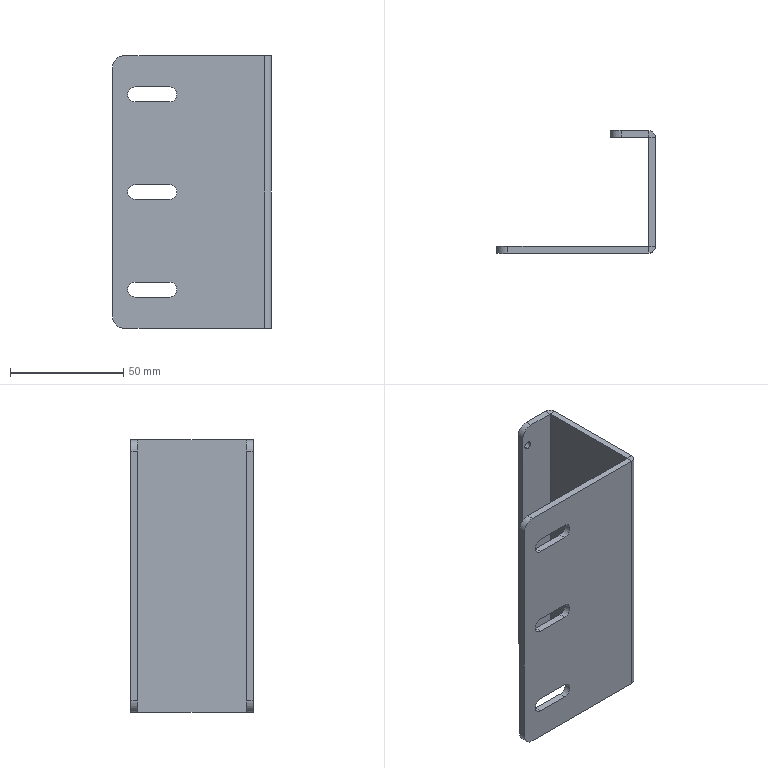Part | SolidWorks | features 3DProfileFeature 1, Fillet 1, FlatPattern 1, HoleWzd 1, ICE 1, SMBaseFlange 1, SheetMetal 1 | 1 solid | 45 faces | box 70 x 54 x 120 mm | volume 47871 mm3 | plane 24 | cylinder 21 | commonest cylinder face diameters 6.6 x9 3.4 x6 10 x4 6 x2
STEP:
#1=CARTESIAN_POINT('',(-17.,51.,8.3));
#2=VERTEX_POINT('',#1);
#3=CARTESIAN_POINT('',(-17.,51.,11.7));
#4=VERTEX_POINT('',#3);
#5=CARTESIAN_POINT('',(-17.,51.,10.));
#6=DIRECTION('',(0.,1.,0.));
#7=DIRECTION('',(0.,0.,1.));
#8=AXIS2_PLACEMENT_3D('',#5,#6,#7);
#9=CIRCLE('',#8,1.7);
#10=EDGE_CURVE('',#2,#4,#9,.T.);
#11=ORIENTED_EDGE('',*,*,#10,.F.);
#12=CARTESIAN_POINT('',(-17.,54.,8.3));
#13=VERTEX_POINT('',#12);
#14=CARTESIAN_POINT('',(-17.,54.,8.3));
#15=DIRECTION('',(0.,1.,0.));
#16=VECTOR('',#15,1000.);
#17=LINE('',#14,#16);
#18=EDGE_CURVE('',#2,#13,#17,.T.);
#19=ORIENTED_EDGE('',*,*,#18,.T.);
#20=CARTESIAN_POINT('',(-17.,54.,11.7));
#21=VERTEX_POINT('',#20);
#22=CARTESIAN_POINT('',(-17.,54.,10.));
#23=DIRECTION('',(0.,1.,0.));
#24=DIRECTION('',(0.,0.,1.));
#25=AXIS2_PLACEMENT_3D('',#22,#23,#24);
#26=CIRCLE('',#25,1.7);
#27=EDGE_CURVE('',#13,#21,#26,.T.);
#28=ORIENTED_EDGE('',*,*,#27,.T.);
#29=CARTESIAN_POINT('',(-17.,54.,11.7));
#30=DIRECTION('',(0.,1.,0.));
#31=VECTOR('',#30,1000.);
#32=LINE('',#29,#31);
#33=EDGE_CURVE('',#4,#21,#32,.T.);
#34=ORIENTED_EDGE('',*,*,#33,.F.);
#35=EDGE_LOOP('',(#11,#19,#28,#34));
#36=FACE_OUTER_BOUND('',#35,.T.);
#37=CARTESIAN_POINT('',(-17.,54.,10.));
#38=DIRECTION('',(0.,1.,0.));
#39=DIRECTION('',(0.,0.,1.));
#40=AXIS2_PLACEMENT_3D('',#37,#38,#39);
#41=CYLINDRICAL_SURFACE('',#40,1.7);
#42=ADVANCED_FACE('',(#36),#41,.F.);
#43=CARTESIAN_POINT('',(-17.,51.,58.3));
#44=VERTEX_POINT('',#43);
#45=CARTESIAN_POINT('',(-17.,51.,61.7));
#46=VERTEX_POINT('',#45);
#47=CARTESIAN_POINT('',(-17.,51.,60.));
#48=DIRECTION('',(0.,1.,0.));
#49=DIRECTION('',(0.,0.,1.));
#50=AXIS2_PLACEMENT_3D('',#47,#48,#49);
#51=CIRCLE('',#50,1.7);
#52=EDGE_CURVE('',#44,#46,#51,.T.);
#53=ORIENTED_EDGE('',*,*,#52,.F.);
#54=CARTESIAN_POINT('',(-17.,54.,58.3));
#55=VERTEX_POINT('',#54);
#56=CARTESIAN_POINT('',(-17.,54.,58.3));
#57=DIRECTION('',(0.,1.,0.));
#58=VECTOR('',#57,1000.);
#59=LINE('',#56,#58);
#60=EDGE_CURVE('',#44,#55,#59,.T.);
#61=ORIENTED_EDGE('',*,*,#60,.T.);
#62=CARTESIAN_POINT('',(-17.,54.,61.7));
#63=VERTEX_POINT('',#62);
#64=CARTESIAN_POINT('',(-17.,54.,60.));
#65=DIRECTION('',(0.,1.,0.));
#66=DIRECTION('',(0.,0.,1.));
#67=AXIS2_PLACEMENT_3D('',#64,#65,#66);
#68=CIRCLE('',#67,1.7);
#69=EDGE_CURVE('',#55,#63,#68,.T.);
#70=ORIENTED_EDGE('',*,*,#69,.T.);
#71=CARTESIAN_POINT('',(-17.,54.,61.7));
#72=DIRECTION('',(0.,1.,0.));
#73=VECTOR('',#72,1000.);
#74=LINE('',#71,#73);
#75=EDGE_CURVE('',#46,#63,#74,.T.);
#76=ORIENTED_EDGE('',*,*,#75,.F.);
#77=EDGE_LOOP('',(#53,#61,#70,#76));
#78=FACE_OUTER_BOUND('',#77,.T.);
#79=CARTESIAN_POINT('',(-17.,54.,60.));
#80=DIRECTION('',(0.,1.,0.));
#81=DIRECTION('',(0.,0.,1.));
#82=AXIS2_PLACEMENT_3D('',#79,#80,#81);
#83=CYLINDRICAL_SURFACE('',#82,1.7);
#84=ADVANCED_FACE('',(#78),#83,.F.);
#85=CARTESIAN_POINT('',(-17.,51.,108.3));
#86=VERTEX_POINT('',#85);
#87=CARTESIAN_POINT('',(-17.,51.,111.7));
#88=VERTEX_POINT('',#87);
#89=CARTESIAN_POINT('',(-17.,51.,110.));
#90=DIRECTION('',(0.,1.,0.));
#91=DIRECTION('',(0.,0.,1.));
#92=AXIS2_PLACEMENT_3D('',#89,#90,#91);
#93=CIRCLE('',#92,1.7);
#94=EDGE_CURVE('',#86,#88,#93,.T.);
#95=ORIENTED_EDGE('',*,*,#94,.F.);
#96=CARTESIAN_POINT('',(-17.,54.,108.3));
#97=VERTEX_POINT('',#96);
#98=CARTESIAN_POINT('',(-17.,54.,108.3));
#99=DIRECTION('',(0.,1.,0.));
#100=VECTOR('',#99,1000.);
#101=LINE('',#98,#100);
#102=EDGE_CURVE('',#86,#97,#101,.T.);
#103=ORIENTED_EDGE('',*,*,#102,.T.);
#104=CARTESIAN_POINT('',(-17.,54.,111.7));
#105=VERTEX_POINT('',#104);
#106=CARTESIAN_POINT('',(-17.,54.,110.));
#107=DIRECTION('',(0.,1.,0.));
#108=DIRECTION('',(0.,0.,1.));
#109=AXIS2_PLACEMENT_3D('',#106,#107,#108);
#110=CIRCLE('',#109,1.7);
#111=EDGE_CURVE('',#97,#105,#110,.T.);
#112=ORIENTED_EDGE('',*,*,#111,.T.);
#113=CARTESIAN_POINT('',(-17.,54.,111.7));
#114=DIRECTION('',(0.,1.,0.));
#115=VECTOR('',#114,1000.);
#116=LINE('',#113,#115);
#117=EDGE_CURVE('',#88,#105,#116,.T.);
#118=ORIENTED_EDGE('',*,*,#117,.F.);
#119=EDGE_LOOP('',(#95,#103,#112,#118));
#120=FACE_OUTER_BOUND('',#119,.T.);
#121=CARTESIAN_POINT('',(-17.,54.,110.));
#122=DIRECTION('',(0.,1.,0.));
#123=DIRECTION('',(0.,0.,1.));
#124=AXIS2_PLACEMENT_3D('',#121,#122,#123);
#125=CYLINDRICAL_SURFACE('',#124,1.7);
#126=ADVANCED_FACE('',(#120),#125,.F.);
#127=CARTESIAN_POINT('',(-63.3,0.,17.));
#128=VERTEX_POINT('',#127);
#129=CARTESIAN_POINT('',(-60.,0.,20.3));
#130=VERTEX_POINT('',#129);
#131=CARTESIAN_POINT('',(-60.,0.,17.));
#132=DIRECTION('',(0.,1.,0.));
#133=DIRECTION('',(-1.,0.,0.));
#134=AXIS2_PLACEMENT_3D('',#131,#132,#133);
#135=CIRCLE('',#134,3.3);
#136=EDGE_CURVE('',#128,#130,#135,.T.);
#137=ORIENTED_EDGE('',*,*,#136,.F.);
#138=CARTESIAN_POINT('',(-63.3,3.,17.));
#139=VERTEX_POINT('',#138);
#140=CARTESIAN_POINT('',(-63.3,0.,17.));
#141=DIRECTION('',(0.,1.,0.));
#142=VECTOR('',#141,1000.);
#143=LINE('',#140,#142);
#144=EDGE_CURVE('',#128,#139,#143,.T.);
#145=ORIENTED_EDGE('',*,*,#144,.T.);
#146=CARTESIAN_POINT('',(-60.,3.,20.3));
#147=VERTEX_POINT('',#146);
#148=CARTESIAN_POINT('',(-60.,3.,17.));
#149=DIRECTION('',(0.,1.,0.));
#150=DIRECTION('',(-1.,0.,0.));
#151=AXIS2_PLACEMENT_3D('',#148,#149,#150);
#152=CIRCLE('',#151,3.3);
#153=EDGE_CURVE('',#139,#147,#152,.T.);
#154=ORIENTED_EDGE('',*,*,#153,.T.);
#155=CARTESIAN_POINT('',(-60.,0.,20.3));
#156=DIRECTION('',(0.,1.,0.));
#157=VECTOR('',#156,1000.);
#158=LINE('',#155,#157);
#159=EDGE_CURVE('',#130,#147,#158,.T.);
#160=ORIENTED_EDGE('',*,*,#159,.F.);
#161=EDGE_LOOP('',(#137,#145,#154,#160));
#162=FACE_OUTER_BOUND('',#161,.T.);
#163=CARTESIAN_POINT('',(-60.,0.,17.));
#164=DIRECTION('',(0.,1.,0.));
#165=DIRECTION('',(-1.,0.,0.));
#166=AXIS2_PLACEMENT_3D('',#163,#164,#165);
#167=CYLINDRICAL_SURFACE('',#166,3.3);
#168=ADVANCED_FACE('',(#162),#167,.F.);
#169=CARTESIAN_POINT('',(-63.3,0.,60.));
#170=VERTEX_POINT('',#169);
#171=CARTESIAN_POINT('',(-60.,0.,63.3));
#172=VERTEX_POINT('',#171);
#173=CARTESIAN_POINT('',(-60.,0.,60.));
#174=DIRECTION('',(0.,1.,0.));
#175=DIRECTION('',(-1.,0.,0.));
#176=AXIS2_PLACEMENT_3D('',#173,#174,#175);
#177=CIRCLE('',#176,3.3);
#178=EDGE_CURVE('',#170,#172,#177,.T.);
#179=ORIENTED_EDGE('',*,*,#178,.F.);
#180=CARTESIAN_POINT('',(-63.3,3.,60.));
#181=VERTEX_POINT('',#180);
#182=CARTESIAN_POINT('',(-63.3,0.,60.));
#183=DIRECTION('',(0.,1.,0.));
#184=VECTOR('',#183,1000.);
#185=LINE('',#182,#184);
#186=EDGE_CURVE('',#170,#181,#185,.T.);
#187=ORIENTED_EDGE('',*,*,#186,.T.);
#188=CARTESIAN_POINT('',(-60.,3.,63.3));
#189=VERTEX_POINT('',#188);
#190=CARTESIAN_POINT('',(-60.,3.,60.));
#191=DIRECTION('',(0.,1.,0.));
#192=DIRECTION('',(-1.,0.,0.));
#193=AXIS2_PLACEMENT_3D('',#190,#191,#192);
#194=CIRCLE('',#193,3.3);
#195=EDGE_CURVE('',#181,#189,#194,.T.);
#196=ORIENTED_EDGE('',*,*,#195,.T.);
#197=CARTESIAN_POINT('',(-60.,0.,63.3));
#198=DIRECTION('',(0.,1.,0.));
#199=VECTOR('',#198,1000.);
#200=LINE('',#197,#199);
#201=EDGE_CURVE('',#172,#189,#200,.T.);
#202=ORIENTED_EDGE('',*,*,#201,.F.);
#203=EDGE_LOOP('',(#179,#187,#196,#202));
#204=FACE_OUTER_BOUND('',#203,.T.);
#205=CARTESIAN_POINT('',(-60.,0.,60.));
#206=DIRECTION('',(0.,1.,0.));
#207=DIRECTION('',(-1.,0.,0.));
#208=AXIS2_PLACEMENT_3D('',#205,#206,#207);
#209=CYLINDRICAL_SURFACE('',#208,3.3);
#210=ADVANCED_FACE('',(#204),#209,.F.);
#211=CARTESIAN_POINT('',(-63.3,0.,103.));
#212=VERTEX_POINT('',#211);
#213=CARTESIAN_POINT('',(-60.,0.,106.3));
#214=VERTEX_POINT('',#213);
#215=CARTESIAN_POINT('',(-60.,0.,103.));
#216=DIRECTION('',(0.,1.,0.));
#217=DIRECTION('',(-1.,0.,0.));
#218=AXIS2_PLACEMENT_3D('',#215,#216,#217);
#219=CIRCLE('',#218,3.3);
#220=EDGE_CURVE('',#212,#214,#219,.T.);
#221=ORIENTED_EDGE('',*,*,#220,.F.);
#222=CARTESIAN_POINT('',(-63.3,3.,103.));
#223=VERTEX_POINT('',#222);
#224=CARTESIAN_POINT('',(-63.3,0.,103.));
#225=DIRECTION('',(0.,1.,0.));
#226=VECTOR('',#225,1000.);
#227=LINE('',#224,#226);
#228=EDGE_CURVE('',#212,#223,#227,.T.);
#229=ORIENTED_EDGE('',*,*,#228,.T.);
#230=CARTESIAN_POINT('',(-60.,3.,106.3));
#231=VERTEX_POINT('',#230);
#232=CARTESIAN_POINT('',(-60.,3.,103.));
#233=DIRECTION('',(0.,1.,0.));
#234=DIRECTION('',(-1.,0.,0.));
#235=AXIS2_PLACEMENT_3D('',#232,#233,#234);
#236=CIRCLE('',#235,3.3);
#237=EDGE_CURVE('',#223,#231,#236,.T.);
#238=ORIENTED_EDGE('',*,*,#237,.T.);
#239=CARTESIAN_POINT('',(-60.,0.,106.3));
#240=DIRECTION('',(0.,1.,0.));
#241=VECTOR('',#240,1000.);
#242=LINE('',#239,#241);
#243=EDGE_CURVE('',#214,#231,#242,.T.);
#244=ORIENTED_EDGE('',*,*,#243,.F.);
#245=EDGE_LOOP('',(#221,#229,#238,#244));
#246=FACE_OUTER_BOUND('',#245,.T.);
#247=CARTESIAN_POINT('',(-60.,0.,103.));
#248=DIRECTION('',(0.,1.,0.));
#249=DIRECTION('',(-1.,0.,0.));
#250=AXIS2_PLACEMENT_3D('',#247,#248,#249);
#251=CYLINDRICAL_SURFACE('',#250,3.3);
#252=ADVANCED_FACE('',(#246),#251,.F.);
#253=CARTESIAN_POINT('',(-3.,51.,120.));
#254=VERTEX_POINT('',#253);
#255=CARTESIAN_POINT('',(0.,51.,120.));
#256=VERTEX_POINT('',#255);
#257=CARTESIAN_POINT('',(-3.,51.,120.));
#258=DIRECTION('',(1.,0.,0.));
#259=VECTOR('',#258,1000.);
#260=LINE('',#257,#259);
#261=EDGE_CURVE('',#254,#256,#260,.T.);
#262=ORIENTED_EDGE('',*,*,#261,.F.);
#263=CARTESIAN_POINT('',(-3.,3.,120.));
#264=VERTEX_POINT('',#263);
#265=CARTESIAN_POINT('',(-3.,0.,120.));
#266=DIRECTION('',(0.,-1.,0.));
#267=VECTOR('',#266,1000.);
#268=LINE('',#265,#267);
#269=EDGE_CURVE('',#254,#264,#268,.T.);
#270=ORIENTED_EDGE('',*,*,#269,.T.);
#271=CARTESIAN_POINT('',(0.,3.,120.));
#272=VERTEX_POINT('',#271);
#273=CARTESIAN_POINT('',(-3.,3.,120.));
#274=DIRECTION('',(1.,0.,0.));
#275=VECTOR('',#274,1000.);
#276=LINE('',#273,#275);
#277=EDGE_CURVE('',#264,#272,#276,.T.);
#278=ORIENTED_EDGE('',*,*,#277,.T.);
#279=CARTESIAN_POINT('',(0.,0.,120.));
#280=DIRECTION('',(0.,-1.,0.));
#281=VECTOR('',#280,1000.);
#282=LINE('',#279,#281);
#283=EDGE_CURVE('',#256,#272,#282,.T.);
#284=ORIENTED_EDGE('',*,*,#283,.F.);
#285=EDGE_LOOP('',(#262,#270,#278,#284));
#286=FACE_OUTER_BOUND('',#285,.T.);
#287=CARTESIAN_POINT('',(-3.,51.,120.));
#288=DIRECTION('',(0.,0.,1.));
#289=DIRECTION('',(1.,0.,0.));
#290=AXIS2_PLACEMENT_3D('',#287,#288,#289);
#291=PLANE('',#290);
#292=ADVANCED_FACE('',(#286),#291,.T.);
#293=CARTESIAN_POINT('',(-3.,54.,120.));
#294=VERTEX_POINT('',#293);
#295=CARTESIAN_POINT('',(-3.,51.,120.));
#296=DIRECTION('',(0.,1.,0.));
#297=VECTOR('',#296,1000.);
#298=LINE('',#295,#297);
#299=EDGE_CURVE('',#254,#294,#298,.T.);
#300=ORIENTED_EDGE('',*,*,#299,.F.);
#301=ORIENTED_EDGE('',*,*,#261,.T.);
#302=CARTESIAN_POINT('',(-3.,51.,120.));
#303=DIRECTION('',(0.,0.,-1.));
#304=DIRECTION('',(1.,0.,0.));
#305=AXIS2_PLACEMENT_3D('',#302,#303,#304);
#306=CIRCLE('',#305,3.);
#307=EDGE_CURVE('',#294,#256,#306,.T.);
#308=ORIENTED_EDGE('',*,*,#307,.F.);
#309=EDGE_LOOP('',(#300,#301,#308));
#310=FACE_OUTER_BOUND('',#309,.T.);
#311=CARTESIAN_POINT('',(-3.,51.,120.));
#312=DIRECTION('',(0.,0.,1.));
#313=DIRECTION('',(1.,0.,0.));
#314=AXIS2_PLACEMENT_3D('',#311,#312,#313);
#315=PLANE('',#314);
#316=ADVANCED_FACE('',(#310),#315,.T.);
#317=CARTESIAN_POINT('',(-15.,51.,0.));
#318=VERTEX_POINT('',#317);
#319=CARTESIAN_POINT('',(-3.,51.,0.));
#320=VERTEX_POINT('',#319);
#321=CARTESIAN_POINT('',(0.,51.,0.));
#322=DIRECTION('',(1.,0.,0.));
#323=VECTOR('',#322,1000.);
#324=LINE('',#321,#323);
#325=EDGE_CURVE('',#318,#320,#324,.T.);
#326=ORIENTED_EDGE('',*,*,#325,.F.);
#327=CARTESIAN_POINT('',(-15.,54.,0.));
#328=VERTEX_POINT('',#327);
#329=CARTESIAN_POINT('',(-15.,51.,0.));
#330=DIRECTION('',(0.,1.,0.));
#331=VECTOR('',#330,1000.);
#332=LINE('',#329,#331);
#333=EDGE_CURVE('',#318,#328,#332,.T.);
#334=ORIENTED_EDGE('',*,*,#333,.T.);
#335=CARTESIAN_POINT('',(-3.,54.,0.));
#336=VERTEX_POINT('',#335);
#337=CARTESIAN_POINT('',(0.,54.,0.));
#338=DIRECTION('',(1.,0.,0.));
#339=VECTOR('',#338,1000.);
#340=LINE('',#337,#339);
#341=EDGE_CURVE('',#328,#336,#340,.T.);
#342=ORIENTED_EDGE('',*,*,#341,.T.);
#343=CARTESIAN_POINT('',(-3.,51.,0.));
#344=DIRECTION('',(0.,1.,0.));
#345=VECTOR('',#344,1000.);
#346=LINE('',#343,#345);
#347=EDGE_CURVE('',#320,#336,#346,.T.);
#348=ORIENTED_EDGE('',*,*,#347,.F.);
#349=EDGE_LOOP('',(#326,#334,#342,#348));
#350=FACE_OUTER_BOUND('',#349,.T.);
#351=CARTESIAN_POINT('',(-3.,51.,0.));
#352=DIRECTION('',(0.,0.,-1.));
#353=DIRECTION('',(-1.,0.,0.));
#354=AXIS2_PLACEMENT_3D('',#351,#352,#353);
#355=PLANE('',#354);
#356=ADVANCED_FACE('',(#350),#355,.T.);
#357=CARTESIAN_POINT('',(0.,51.,0.));
#358=VERTEX_POINT('',#357);
#359=CARTESIAN_POINT('',(-3.,51.,0.));
#360=DIRECTION('',(1.,0.,0.));
#361=VECTOR('',#360,1000.);
#362=LINE('',#359,#361);
#363=EDGE_CURVE('',#320,#358,#362,.T.);
#364=ORIENTED_EDGE('',*,*,#363,.F.);
#365=ORIENTED_EDGE('',*,*,#347,.T.);
#366=CARTESIAN_POINT('',(-3.,51.,0.));
#367=DIRECTION('',(0.,0.,-1.));
#368=DIRECTION('',(1.,0.,0.));
#369=AXIS2_PLACEMENT_3D('',#366,#367,#368);
#370=CIRCLE('',#369,3.);
#371=EDGE_CURVE('',#336,#358,#370,.T.);
#372=ORIENTED_EDGE('',*,*,#371,.T.);
#373=EDGE_LOOP('',(#364,#365,#372));
#374=FACE_OUTER_BOUND('',#373,.T.);
#375=CARTESIAN_POINT('',(-3.,51.,0.));
#376=DIRECTION('',(0.,0.,-1.));
#377=DIRECTION('',(-1.,0.,0.));
#378=AXIS2_PLACEMENT_3D('',#375,#376,#377);
#379=PLANE('',#378);
#380=ADVANCED_FACE('',(#374),#379,.T.);
#381=CARTESIAN_POINT('',(-65.,3.,120.));
#382=VERTEX_POINT('',#381);
#383=CARTESIAN_POINT('',(0.,3.,120.));
#384=DIRECTION('',(-1.,0.,0.));
#385=VECTOR('',#384,1000.);
#386=LINE('',#383,#385);
#387=EDGE_CURVE('',#264,#382,#386,.T.);
#388=ORIENTED_EDGE('',*,*,#387,.T.);
#389=CARTESIAN_POINT('',(-65.,0.,120.));
#390=VERTEX_POINT('',#389);
#391=CARTESIAN_POINT('',(-65.,3.,120.));
#392=DIRECTION('',(0.,-1.,0.));
#393=VECTOR('',#392,1000.);
#394=LINE('',#391,#393);
#395=EDGE_CURVE('',#382,#390,#394,.T.);
#396=ORIENTED_EDGE('',*,*,#395,.T.);
#397=CARTESIAN_POINT('',(-3.,0.,120.));
#398=VERTEX_POINT('',#397);
#399=CARTESIAN_POINT('',(0.,0.,120.));
#400=DIRECTION('',(-1.,0.,0.));
#401=VECTOR('',#400,1000.);
#402=LINE('',#399,#401);
#403=EDGE_CURVE('',#398,#390,#402,.T.);
#404=ORIENTED_EDGE('',*,*,#403,.F.);
#405=CARTESIAN_POINT('',(-3.,3.,120.));
#406=DIRECTION('',(0.,-1.,0.));
#407=VECTOR('',#406,1000.);
#408=LINE('',#405,#407);
#409=EDGE_CURVE('',#264,#398,#408,.T.);
#410=ORIENTED_EDGE('',*,*,#409,.F.);
#411=EDGE_LOOP('',(#388,#396,#404,#410));
#412=FACE_OUTER_BOUND('',#411,.T.);
#413=CARTESIAN_POINT('',(-3.,3.,120.));
#414=DIRECTION('',(0.,0.,1.));
#415=DIRECTION('',(1.,0.,0.));
#416=AXIS2_PLACEMENT_3D('',#413,#414,#415);
#417=PLANE('',#416);
#418=ADVANCED_FACE('',(#412),#417,.T.);
#419=ORIENTED_EDGE('',*,*,#277,.F.);
#420=ORIENTED_EDGE('',*,*,#409,.T.);
#421=CARTESIAN_POINT('',(-3.,3.,120.));
#422=DIRECTION('',(0.,0.,-1.));
#423=DIRECTION('',(1.,0.,0.));
#424=AXIS2_PLACEMENT_3D('',#421,#422,#423);
#425=CIRCLE('',#424,3.);
#426=EDGE_CURVE('',#272,#398,#425,.T.);
#427=ORIENTED_EDGE('',*,*,#426,.F.);
#428=EDGE_LOOP('',(#419,#420,#427));
#429=FACE_OUTER_BOUND('',#428,.T.);
#430=CARTESIAN_POINT('',(-3.,3.,120.));
#431=DIRECTION('',(0.,0.,1.));
#432=DIRECTION('',(1.,0.,0.));
#433=AXIS2_PLACEMENT_3D('',#430,#431,#432);
#434=PLANE('',#433);
#435=ADVANCED_FACE('',(#429),#434,.T.);
#436=CARTESIAN_POINT('',(-3.,3.,0.));
#437=VERTEX_POINT('',#436);
#438=CARTESIAN_POINT('',(0.,3.,0.));
#439=VERTEX_POINT('',#438);
#440=CARTESIAN_POINT('',(-3.,3.,0.));
#441=DIRECTION('',(1.,0.,0.));
#442=VECTOR('',#441,1000.);
#443=LINE('',#440,#442);
#444=EDGE_CURVE('',#437,#439,#443,.T.);
#445=ORIENTED_EDGE('',*,*,#444,.F.);
#446=CARTESIAN_POINT('',(-3.,0.,0.));
#447=DIRECTION('',(0.,-1.,0.));
#448=VECTOR('',#447,1000.);
#449=LINE('',#446,#448);
#450=EDGE_CURVE('',#320,#437,#449,.T.);
#451=ORIENTED_EDGE('',*,*,#450,.F.);
#452=ORIENTED_EDGE('',*,*,#363,.T.);
#453=CARTESIAN_POINT('',(0.,0.,0.));
#454=DIRECTION('',(0.,-1.,0.));
#455=VECTOR('',#454,1000.);
#456=LINE('',#453,#455);
#457=EDGE_CURVE('',#358,#439,#456,.T.);
#458=ORIENTED_EDGE('',*,*,#457,.T.);
#459=EDGE_LOOP('',(#445,#451,#452,#458));
#460=FACE_OUTER_BOUND('',#459,.T.);
#461=CARTESIAN_POINT('',(-3.,3.,0.));
#462=DIRECTION('',(0.,0.,-1.));
#463=DIRECTION('',(-1.,0.,0.));
#464=AXIS2_PLACEMENT_3D('',#461,#462,#463);
#465=PLANE('',#464);
#466=ADVANCED_FACE('',(#460),#465,.T.);
#467=CARTESIAN_POINT('',(-3.,0.,0.));
#468=VERTEX_POINT('',#467);
#469=CARTESIAN_POINT('',(-3.,3.,0.));
#470=DIRECTION('',(0.,-1.,0.));
#471=VECTOR('',#470,1000.);
#472=LINE('',#469,#471);
#473=EDGE_CURVE('',#437,#468,#472,.T.);
#474=ORIENTED_EDGE('',*,*,#473,.F.);
#475=ORIENTED_EDGE('',*,*,#444,.T.);
#476=CARTESIAN_POINT('',(-3.,3.,0.));
#477=DIRECTION('',(0.,0.,-1.));
#478=DIRECTION('',(1.,0.,0.));
#479=AXIS2_PLACEMENT_3D('',#476,#477,#478);
#480=CIRCLE('',#479,3.);
#481=EDGE_CURVE('',#439,#468,#480,.T.);
#482=ORIENTED_EDGE('',*,*,#481,.T.);
#483=EDGE_LOOP('',(#474,#475,#482));
#484=FACE_OUTER_BOUND('',#483,.T.);
#485=CARTESIAN_POINT('',(-3.,3.,0.));
#486=DIRECTION('',(0.,0.,-1.));
#487=DIRECTION('',(-1.,0.,0.));
#488=AXIS2_PLACEMENT_3D('',#485,#486,#487);
#489=PLANE('',#488);
#490=ADVANCED_FACE('',(#484),#489,.T.);
#491=CARTESIAN_POINT('',(-45.,3.,20.3));
#492=VERTEX_POINT('',#491);
#493=CARTESIAN_POINT('',(-60.,3.,20.3));
#494=DIRECTION('',(1.,0.,0.));
#495=VECTOR('',#494,1000.);
#496=LINE('',#493,#495);
#497=EDGE_CURVE('',#147,#492,#496,.T.);
#498=ORIENTED_EDGE('',*,*,#497,.F.);
#499=ORIENTED_EDGE('',*,*,#153,.F.);
#500=CARTESIAN_POINT('',(-60.,3.,13.7));
#501=VERTEX_POINT('',#500);
#502=CARTESIAN_POINT('',(-60.,3.,17.));
#503=DIRECTION('',(0.,1.,0.));
#504=DIRECTION('',(-1.,0.,0.));
#505=AXIS2_PLACEMENT_3D('',#502,#503,#504);
#506=CIRCLE('',#505,3.3);
#507=EDGE_CURVE('',#501,#139,#506,.T.);
#508=ORIENTED_EDGE('',*,*,#507,.F.);
#509=CARTESIAN_POINT('',(-45.,3.,13.7));
#510=VERTEX_POINT('',#509);
#511=CARTESIAN_POINT('',(-60.,3.,13.7));
#512=DIRECTION('',(-1.,0.,0.));
#513=VECTOR('',#512,1000.);
#514=LINE('',#511,#513);
#515=EDGE_CURVE('',#510,#501,#514,.T.);
#516=ORIENTED_EDGE('',*,*,#515,.F.);
#517=CARTESIAN_POINT('',(-45.,3.,17.));
#518=DIRECTION('',(0.,1.,0.));
#519=DIRECTION('',(-1.,0.,0.));
#520=AXIS2_PLACEMENT_3D('',#517,#518,#519);
#521=CIRCLE('',#520,3.3);
#522=EDGE_CURVE('',#492,#510,#521,.T.);
#523=ORIENTED_EDGE('',*,*,#522,.F.);
#524=EDGE_LOOP('',(#498,#499,#508,#516,#523));
#525=FACE_BOUND('',#524,.T.);
#526=CARTESIAN_POINT('',(-45.,3.,63.3));
#527=VERTEX_POINT('',#526);
#528=CARTESIAN_POINT('',(-60.,3.,63.3));
#529=DIRECTION('',(1.,0.,0.));
#530=VECTOR('',#529,1000.);
#531=LINE('',#528,#530);
#532=EDGE_CURVE('',#189,#527,#531,.T.);
#533=ORIENTED_EDGE('',*,*,#532,.F.);
#534=ORIENTED_EDGE('',*,*,#195,.F.);
#535=CARTESIAN_POINT('',(-60.,3.,56.7));
#536=VERTEX_POINT('',#535);
#537=CARTESIAN_POINT('',(-60.,3.,60.));
#538=DIRECTION('',(0.,1.,0.));
#539=DIRECTION('',(-1.,0.,0.));
#540=AXIS2_PLACEMENT_3D('',#537,#538,#539);
#541=CIRCLE('',#540,3.3);
#542=EDGE_CURVE('',#536,#181,#541,.T.);
#543=ORIENTED_EDGE('',*,*,#542,.F.);
#544=CARTESIAN_POINT('',(-45.,3.,56.7));
#545=VERTEX_POINT('',#544);
#546=CARTESIAN_POINT('',(-60.,3.,56.7));
#547=DIRECTION('',(-1.,0.,0.));
#548=VECTOR('',#547,1000.);
#549=LINE('',#546,#548);
#550=EDGE_CURVE('',#545,#536,#549,.T.);
#551=ORIENTED_EDGE('',*,*,#550,.F.);
#552=CARTESIAN_POINT('',(-45.,3.,60.));
#553=DIRECTION('',(0.,1.,0.));
#554=DIRECTION('',(-1.,0.,0.));
#555=AXIS2_PLACEMENT_3D('',#552,#553,#554);
#556=CIRCLE('',#555,3.3);
#557=EDGE_CURVE('',#527,#545,#556,.T.);
#558=ORIENTED_EDGE('',*,*,#557,.F.);
#559=EDGE_LOOP('',(#533,#534,#543,#551,#558));
#560=FACE_BOUND('',#559,.T.);
#561=CARTESIAN_POINT('',(-45.,3.,106.3));
#562=VERTEX_POINT('',#561);
#563=CARTESIAN_POINT('',(-60.,3.,106.3));
#564=DIRECTION('',(1.,0.,0.));
#565=VECTOR('',#564,1000.);
#566=LINE('',#563,#565);
#567=EDGE_CURVE('',#231,#562,#566,.T.);
#568=ORIENTED_EDGE('',*,*,#567,.F.);
#569=ORIENTED_EDGE('',*,*,#237,.F.);
#570=CARTESIAN_POINT('',(-60.,3.,99.7));
#571=VERTEX_POINT('',#570);
#572=CARTESIAN_POINT('',(-60.,3.,103.));
#573=DIRECTION('',(0.,1.,0.));
#574=DIRECTION('',(-1.,0.,0.));
#575=AXIS2_PLACEMENT_3D('',#572,#573,#574);
#576=CIRCLE('',#575,3.3);
#577=EDGE_CURVE('',#571,#223,#576,.T.);
#578=ORIENTED_EDGE('',*,*,#577,.F.);
#579=CARTESIAN_POINT('',(-45.,3.,99.7));
#580=VERTEX_POINT('',#579);
#581=CARTESIAN_POINT('',(-60.,3.,99.7));
#582=DIRECTION('',(-1.,0.,0.));
#583=VECTOR('',#582,1000.);
#584=LINE('',#581,#583);
#585=EDGE_CURVE('',#580,#571,#584,.T.);
#586=ORIENTED_EDGE('',*,*,#585,.F.);
#587=CARTESIAN_POINT('',(-45.,3.,103.));
#588=DIRECTION('',(0.,1.,0.));
#589=DIRECTION('',(-1.,0.,0.));
#590=AXIS2_PLACEMENT_3D('',#587,#588,#589);
#591=CIRCLE('',#590,3.3);
#592=EDGE_CURVE('',#562,#580,#591,.T.);
#593=ORIENTED_EDGE('',*,*,#592,.F.);
#594=EDGE_LOOP('',(#568,#569,#578,#586,#593));
#595=FACE_BOUND('',#594,.T.);
#596=CARTESIAN_POINT('',(-65.,3.,0.));
#597=VERTEX_POINT('',#596);
#598=CARTESIAN_POINT('',(0.,3.,0.));
#599=DIRECTION('',(-1.,0.,0.));
#600=VECTOR('',#599,1000.);
#601=LINE('',#598,#600);
#602=EDGE_CURVE('',#437,#597,#601,.T.);
#603=ORIENTED_EDGE('',*,*,#602,.T.);
#604=CARTESIAN_POINT('',(-70.,3.,5.));
#605=VERTEX_POINT('',#604);
#606=CARTESIAN_POINT('',(-65.,3.,5.));
#607=DIRECTION('',(0.,1.,0.));
#608=DIRECTION('',(1.,0.,0.));
#609=AXIS2_PLACEMENT_3D('',#606,#607,#608);
#610=CIRCLE('',#609,5.);
#611=EDGE_CURVE('',#597,#605,#610,.T.);
#612=ORIENTED_EDGE('',*,*,#611,.T.);
#613=CARTESIAN_POINT('',(-70.,3.,115.));
#614=VERTEX_POINT('',#613);
#615=CARTESIAN_POINT('',(-70.,3.,120.));
#616=DIRECTION('',(0.,0.,-1.));
#617=VECTOR('',#616,1000.);
#618=LINE('',#615,#617);
#619=EDGE_CURVE('',#614,#605,#618,.T.);
#620=ORIENTED_EDGE('',*,*,#619,.F.);
#621=CARTESIAN_POINT('',(-65.,3.,115.));
#622=DIRECTION('',(0.,1.,0.));
#623=DIRECTION('',(1.,0.,0.));
#624=AXIS2_PLACEMENT_3D('',#621,#622,#623);
#625=CIRCLE('',#624,5.);
#626=EDGE_CURVE('',#614,#382,#625,.T.);
#627=ORIENTED_EDGE('',*,*,#626,.T.);
#628=ORIENTED_EDGE('',*,*,#387,.F.);
#629=CARTESIAN_POINT('',(-3.,3.,120.));
#630=DIRECTION('',(0.,0.,-1.));
#631=VECTOR('',#630,1000.);
#632=LINE('',#629,#631);
#633=EDGE_CURVE('',#264,#437,#632,.T.);
#634=ORIENTED_EDGE('',*,*,#633,.T.);
#635=EDGE_LOOP('',(#603,#612,#620,#627,#628,#634));
#636=FACE_OUTER_BOUND('',#635,.T.);
#637=CARTESIAN_POINT('',(0.,3.,120.));
#638=DIRECTION('',(0.,-1.,0.));
#639=DIRECTION('',(1.,0.,0.));
#640=AXIS2_PLACEMENT_3D('',#637,#638,#639);
#641=PLANE('',#640);
#642=ADVANCED_FACE('',(#525,#560,#595,#636),#641,.F.);
#643=ORIENTED_EDGE('',*,*,#619,.T.);
#644=CARTESIAN_POINT('',(-70.,0.,5.));
#645=VERTEX_POINT('',#644);
#646=CARTESIAN_POINT('',(-70.,0.,5.));
#647=DIRECTION('',(0.,-1.,0.));
#648=VECTOR('',#647,1000.);
#649=LINE('',#646,#648);
#650=EDGE_CURVE('',#605,#645,#649,.T.);
#651=ORIENTED_EDGE('',*,*,#650,.T.);
#652=CARTESIAN_POINT('',(-70.,0.,115.));
#653=VERTEX_POINT('',#652);
#654=CARTESIAN_POINT('',(-70.,0.,120.));
#655=DIRECTION('',(0.,0.,-1.));
#656=VECTOR('',#655,1000.);
#657=LINE('',#654,#656);
#658=EDGE_CURVE('',#653,#645,#657,.T.);
#659=ORIENTED_EDGE('',*,*,#658,.F.);
#660=CARTESIAN_POINT('',(-70.,0.,115.));
#661=DIRECTION('',(0.,1.,0.));
#662=VECTOR('',#661,1000.);
#663=LINE('',#660,#662);
#664=EDGE_CURVE('',#653,#614,#663,.T.);
#665=ORIENTED_EDGE('',*,*,#664,.T.);
#666=EDGE_LOOP('',(#643,#651,#659,#665));
#667=FACE_OUTER_BOUND('',#666,.T.);
#668=CARTESIAN_POINT('',(-70.,0.,120.));
#669=DIRECTION('',(-1.,0.,0.));
#670=DIRECTION('',(0.,0.,1.));
#671=AXIS2_PLACEMENT_3D('',#668,#669,#670);
#672=PLANE('',#671);
#673=ADVANCED_FACE('',(#667),#672,.T.);
#674=CARTESIAN_POINT('',(-60.,0.,13.7));
#675=VERTEX_POINT('',#674);
#676=CARTESIAN_POINT('',(-60.,0.,17.));
#677=DIRECTION('',(0.,1.,0.));
#678=DIRECTION('',(-1.,0.,0.));
#679=AXIS2_PLACEMENT_3D('',#676,#677,#678);
#680=CIRCLE('',#679,3.3);
#681=EDGE_CURVE('',#675,#128,#680,.T.);
#682=ORIENTED_EDGE('',*,*,#681,.T.);
#683=ORIENTED_EDGE('',*,*,#136,.T.);
#684=CARTESIAN_POINT('',(-45.,0.,20.3));
#685=VERTEX_POINT('',#684);
#686=CARTESIAN_POINT('',(-60.,0.,20.3));
#687=DIRECTION('',(1.,0.,0.));
#688=VECTOR('',#687,1000.);
#689=LINE('',#686,#688);
#690=EDGE_CURVE('',#130,#685,#689,.T.);
#691=ORIENTED_EDGE('',*,*,#690,.T.);
#692=CARTESIAN_POINT('',(-45.,0.,13.7));
#693=VERTEX_POINT('',#692);
#694=CARTESIAN_POINT('',(-45.,0.,17.));
#695=DIRECTION('',(0.,1.,0.));
#696=DIRECTION('',(-1.,0.,0.));
#697=AXIS2_PLACEMENT_3D('',#694,#695,#696);
#698=CIRCLE('',#697,3.3);
#699=EDGE_CURVE('',#685,#693,#698,.T.);
#700=ORIENTED_EDGE('',*,*,#699,.T.);
#701=CARTESIAN_POINT('',(-60.,0.,13.7));
#702=DIRECTION('',(-1.,0.,0.));
#703=VECTOR('',#702,1000.);
#704=LINE('',#701,#703);
#705=EDGE_CURVE('',#693,#675,#704,.T.);
#706=ORIENTED_EDGE('',*,*,#705,.T.);
#707=EDGE_LOOP('',(#682,#683,#691,#700,#706));
#708=FACE_BOUND('',#707,.T.);
#709=CARTESIAN_POINT('',(-60.,0.,56.7));
#710=VERTEX_POINT('',#709);
#711=CARTESIAN_POINT('',(-60.,0.,60.));
#712=DIRECTION('',(0.,1.,0.));
#713=DIRECTION('',(-1.,0.,0.));
#714=AXIS2_PLACEMENT_3D('',#711,#712,#713);
#715=CIRCLE('',#714,3.3);
#716=EDGE_CURVE('',#710,#170,#715,.T.);
#717=ORIENTED_EDGE('',*,*,#716,.T.);
#718=ORIENTED_EDGE('',*,*,#178,.T.);
#719=CARTESIAN_POINT('',(-45.,0.,63.3));
#720=VERTEX_POINT('',#719);
#721=CARTESIAN_POINT('',(-60.,0.,63.3));
#722=DIRECTION('',(1.,0.,0.));
#723=VECTOR('',#722,1000.);
#724=LINE('',#721,#723);
#725=EDGE_CURVE('',#172,#720,#724,.T.);
#726=ORIENTED_EDGE('',*,*,#725,.T.);
#727=CARTESIAN_POINT('',(-45.,0.,56.7));
#728=VERTEX_POINT('',#727);
#729=CARTESIAN_POINT('',(-45.,0.,60.));
#730=DIRECTION('',(0.,1.,0.));
#731=DIRECTION('',(-1.,0.,0.));
#732=AXIS2_PLACEMENT_3D('',#729,#730,#731);
#733=CIRCLE('',#732,3.3);
#734=EDGE_CURVE('',#720,#728,#733,.T.);
#735=ORIENTED_EDGE('',*,*,#734,.T.);
#736=CARTESIAN_POINT('',(-60.,0.,56.7));
#737=DIRECTION('',(-1.,0.,0.));
#738=VECTOR('',#737,1000.);
#739=LINE('',#736,#738);
#740=EDGE_CURVE('',#728,#710,#739,.T.);
#741=ORIENTED_EDGE('',*,*,#740,.T.);
#742=EDGE_LOOP('',(#717,#718,#726,#735,#741));
#743=FACE_BOUND('',#742,.T.);
#744=CARTESIAN_POINT('',(-60.,0.,99.7));
#745=VERTEX_POINT('',#744);
#746=CARTESIAN_POINT('',(-60.,0.,103.));
#747=DIRECTION('',(0.,1.,0.));
#748=DIRECTION('',(-1.,0.,0.));
#749=AXIS2_PLACEMENT_3D('',#746,#747,#748);
#750=CIRCLE('',#749,3.3);
#751=EDGE_CURVE('',#745,#212,#750,.T.);
#752=ORIENTED_EDGE('',*,*,#751,.T.);
#753=ORIENTED_EDGE('',*,*,#220,.T.);
#754=CARTESIAN_POINT('',(-45.,0.,106.3));
#755=VERTEX_POINT('',#754);
#756=CARTESIAN_POINT('',(-60.,0.,106.3));
#757=DIRECTION('',(1.,0.,0.));
#758=VECTOR('',#757,1000.);
#759=LINE('',#756,#758);
#760=EDGE_CURVE('',#214,#755,#759,.T.);
#761=ORIENTED_EDGE('',*,*,#760,.T.);
#762=CARTESIAN_POINT('',(-45.,0.,99.7));
#763=VERTEX_POINT('',#762);
#764=CARTESIAN_POINT('',(-45.,0.,103.));
#765=DIRECTION('',(0.,1.,0.));
#766=DIRECTION('',(-1.,0.,0.));
#767=AXIS2_PLACEMENT_3D('',#764,#765,#766);
#768=CIRCLE('',#767,3.3);
#769=EDGE_CURVE('',#755,#763,#768,.T.);
#770=ORIENTED_EDGE('',*,*,#769,.T.);
#771=CARTESIAN_POINT('',(-60.,0.,99.7));
#772=DIRECTION('',(-1.,0.,0.));
#773=VECTOR('',#772,1000.);
#774=LINE('',#771,#773);
#775=EDGE_CURVE('',#763,#745,#774,.T.);
#776=ORIENTED_EDGE('',*,*,#775,.T.);
#777=EDGE_LOOP('',(#752,#753,#761,#770,#776));
#778=FACE_BOUND('',#777,.T.);
#779=ORIENTED_EDGE('',*,*,#658,.T.);
#780=CARTESIAN_POINT('',(-65.,0.,0.));
#781=VERTEX_POINT('',#780);
#782=CARTESIAN_POINT('',(-65.,0.,5.));
#783=DIRECTION('',(0.,-1.,0.));
#784=DIRECTION('',(1.,0.,0.));
#785=AXIS2_PLACEMENT_3D('',#782,#783,#784);
#786=CIRCLE('',#785,5.);
#787=EDGE_CURVE('',#645,#781,#786,.T.);
#788=ORIENTED_EDGE('',*,*,#787,.T.);
#789=CARTESIAN_POINT('',(0.,0.,0.));
#790=DIRECTION('',(-1.,0.,0.));
#791=VECTOR('',#790,1000.);
#792=LINE('',#789,#791);
#793=EDGE_CURVE('',#468,#781,#792,.T.);
#794=ORIENTED_EDGE('',*,*,#793,.F.);
#795=CARTESIAN_POINT('',(-3.,0.,120.));
#796=DIRECTION('',(0.,0.,-1.));
#797=VECTOR('',#796,1000.);
#798=LINE('',#795,#797);
#799=EDGE_CURVE('',#398,#468,#798,.T.);
#800=ORIENTED_EDGE('',*,*,#799,.F.);
#801=ORIENTED_EDGE('',*,*,#403,.T.);
#802=CARTESIAN_POINT('',(-65.,0.,115.));
#803=DIRECTION('',(0.,-1.,0.));
#804=DIRECTION('',(1.,0.,0.));
#805=AXIS2_PLACEMENT_3D('',#802,#803,#804);
#806=CIRCLE('',#805,5.);
#807=EDGE_CURVE('',#390,#653,#806,.T.);
#808=ORIENTED_EDGE('',*,*,#807,.T.);
#809=EDGE_LOOP('',(#779,#788,#794,#800,#801,#808));
#810=FACE_OUTER_BOUND('',#809,.T.);
#811=CARTESIAN_POINT('',(0.,0.,120.));
#812=DIRECTION('',(0.,-1.,0.));
#813=DIRECTION('',(1.,0.,0.));
#814=AXIS2_PLACEMENT_3D('',#811,#812,#813);
#815=PLANE('',#814);
#816=ADVANCED_FACE('',(#708,#743,#778,#810),#815,.T.);
#817=ORIENTED_EDGE('',*,*,#481,.F.);
#818=CARTESIAN_POINT('',(0.,3.,120.));
#819=DIRECTION('',(0.,0.,-1.));
#820=VECTOR('',#819,1000.);
#821=LINE('',#818,#820);
#822=EDGE_CURVE('',#272,#439,#821,.T.);
#823=ORIENTED_EDGE('',*,*,#822,.F.);
#824=ORIENTED_EDGE('',*,*,#426,.T.);
#825=ORIENTED_EDGE('',*,*,#799,.T.);
#826=EDGE_LOOP('',(#817,#823,#824,#825));
#827=FACE_OUTER_BOUND('',#826,.T.);
#828=CARTESIAN_POINT('',(-3.,3.,120.));
#829=DIRECTION('',(0.,0.,-1.));
#830=DIRECTION('',(-1.,0.,0.));
#831=AXIS2_PLACEMENT_3D('',#828,#829,#830);
#832=CYLINDRICAL_SURFACE('',#831,3.);
#833=ADVANCED_FACE('',(#827),#832,.T.);
#834=ORIENTED_EDGE('',*,*,#457,.F.);
#835=CARTESIAN_POINT('',(0.,51.,120.));
#836=DIRECTION('',(0.,0.,-1.));
#837=VECTOR('',#836,1000.);
#838=LINE('',#835,#837);
#839=EDGE_CURVE('',#256,#358,#838,.T.);
#840=ORIENTED_EDGE('',*,*,#839,.F.);
#841=ORIENTED_EDGE('',*,*,#283,.T.);
#842=ORIENTED_EDGE('',*,*,#822,.T.);
#843=EDGE_LOOP('',(#834,#840,#841,#842));
#844=FACE_OUTER_BOUND('',#843,.T.);
#845=CARTESIAN_POINT('',(0.,0.,120.));
#846=DIRECTION('',(1.,0.,0.));
#847=DIRECTION('',(0.,0.,-1.));
#848=AXIS2_PLACEMENT_3D('',#845,#846,#847);
#849=PLANE('',#848);
#850=ADVANCED_FACE('',(#844),#849,.T.);
#851=ORIENTED_EDGE('',*,*,#371,.F.);
#852=CARTESIAN_POINT('',(-3.,54.,120.));
#853=DIRECTION('',(0.,0.,-1.));
#854=VECTOR('',#853,1000.);
#855=LINE('',#852,#854);
#856=EDGE_CURVE('',#294,#336,#855,.T.);
#857=ORIENTED_EDGE('',*,*,#856,.F.);
#858=ORIENTED_EDGE('',*,*,#307,.T.);
#859=ORIENTED_EDGE('',*,*,#839,.T.);
#860=EDGE_LOOP('',(#851,#857,#858,#859));
#861=FACE_OUTER_BOUND('',#860,.T.);
#862=CARTESIAN_POINT('',(-3.,51.,120.));
#863=DIRECTION('',(0.,0.,-1.));
#864=DIRECTION('',(-1.,0.,0.));
#865=AXIS2_PLACEMENT_3D('',#862,#863,#864);
#866=CYLINDRICAL_SURFACE('',#865,3.);
#867=ADVANCED_FACE('',(#861),#866,.T.);
#868=CARTESIAN_POINT('',(-17.,54.,10.));
#869=DIRECTION('',(0.,1.,0.));
#870=DIRECTION('',(0.,0.,1.));
#871=AXIS2_PLACEMENT_3D('',#868,#869,#870);
#872=CIRCLE('',#871,1.7);
#873=EDGE_CURVE('',#21,#13,#872,.T.);
#874=ORIENTED_EDGE('',*,*,#873,.F.);
#875=ORIENTED_EDGE('',*,*,#27,.F.);
#876=EDGE_LOOP('',(#874,#875));
#877=FACE_BOUND('',#876,.T.);
#878=CARTESIAN_POINT('',(-17.,54.,60.));
#879=DIRECTION('',(0.,1.,0.));
#880=DIRECTION('',(0.,0.,1.));
#881=AXIS2_PLACEMENT_3D('',#878,#879,#880);
#882=CIRCLE('',#881,1.7);
#883=EDGE_CURVE('',#63,#55,#882,.T.);
#884=ORIENTED_EDGE('',*,*,#883,.F.);
#885=ORIENTED_EDGE('',*,*,#69,.F.);
#886=EDGE_LOOP('',(#884,#885));
#887=FACE_BOUND('',#886,.T.);
#888=CARTESIAN_POINT('',(-17.,54.,110.));
#889=DIRECTION('',(0.,1.,0.));
#890=DIRECTION('',(0.,0.,1.));
#891=AXIS2_PLACEMENT_3D('',#888,#889,#890);
#892=CIRCLE('',#891,1.7);
#893=EDGE_CURVE('',#105,#97,#892,.T.);
#894=ORIENTED_EDGE('',*,*,#893,.F.);
#895=ORIENTED_EDGE('',*,*,#111,.F.);
#896=EDGE_LOOP('',(#894,#895));
#897=FACE_BOUND('',#896,.T.);
#898=ORIENTED_EDGE('',*,*,#341,.F.);
#899=CARTESIAN_POINT('',(-20.,54.,5.));
#900=VERTEX_POINT('',#899);
#901=CARTESIAN_POINT('',(-15.,54.,5.));
#902=DIRECTION('',(0.,1.,0.));
#903=DIRECTION('',(0.,0.,1.));
#904=AXIS2_PLACEMENT_3D('',#901,#902,#903);
#905=CIRCLE('',#904,5.);
#906=EDGE_CURVE('',#328,#900,#905,.T.);
#907=ORIENTED_EDGE('',*,*,#906,.T.);
#908=CARTESIAN_POINT('',(-20.,54.,115.));
#909=VERTEX_POINT('',#908);
#910=CARTESIAN_POINT('',(-20.,54.,120.));
#911=DIRECTION('',(0.,0.,-1.));
#912=VECTOR('',#911,1000.);
#913=LINE('',#910,#912);
#914=EDGE_CURVE('',#909,#900,#913,.T.);
#915=ORIENTED_EDGE('',*,*,#914,.F.);
#916=CARTESIAN_POINT('',(-15.,54.,120.));
#917=VERTEX_POINT('',#916);
#918=CARTESIAN_POINT('',(-15.,54.,115.));
#919=DIRECTION('',(0.,1.,0.));
#920=DIRECTION('',(0.,0.,1.));
#921=AXIS2_PLACEMENT_3D('',#918,#919,#920);
#922=CIRCLE('',#921,5.);
#923=EDGE_CURVE('',#909,#917,#922,.T.);
#924=ORIENTED_EDGE('',*,*,#923,.T.);
#925=CARTESIAN_POINT('',(0.,54.,120.));
#926=DIRECTION('',(1.,0.,0.));
#927=VECTOR('',#926,1000.);
#928=LINE('',#925,#927);
#929=EDGE_CURVE('',#917,#294,#928,.T.);
#930=ORIENTED_EDGE('',*,*,#929,.T.);
#931=ORIENTED_EDGE('',*,*,#856,.T.);
#932=EDGE_LOOP('',(#898,#907,#915,#924,#930,#931));
#933=FACE_OUTER_BOUND('',#932,.T.);
#934=CARTESIAN_POINT('',(0.,54.,120.));
#935=DIRECTION('',(0.,1.,0.));
#936=DIRECTION('',(0.,0.,1.));
#937=AXIS2_PLACEMENT_3D('',#934,#935,#936);
#938=PLANE('',#937);
#939=ADVANCED_FACE('',(#877,#887,#897,#933),#938,.T.);
#940=ORIENTED_EDGE('',*,*,#914,.T.);
#941=CARTESIAN_POINT('',(-20.,51.,5.));
#942=VERTEX_POINT('',#941);
#943=CARTESIAN_POINT('',(-20.,51.,5.));
#944=DIRECTION('',(0.,-1.,0.));
#945=VECTOR('',#944,1000.);
#946=LINE('',#943,#945);
#947=EDGE_CURVE('',#900,#942,#946,.T.);
#948=ORIENTED_EDGE('',*,*,#947,.T.);
#949=CARTESIAN_POINT('',(-20.,51.,115.));
#950=VERTEX_POINT('',#949);
#951=CARTESIAN_POINT('',(-20.,51.,120.));
#952=DIRECTION('',(0.,0.,-1.));
#953=VECTOR('',#952,1000.);
#954=LINE('',#951,#953);
#955=EDGE_CURVE('',#950,#942,#954,.T.);
#956=ORIENTED_EDGE('',*,*,#955,.F.);
#957=CARTESIAN_POINT('',(-20.,51.,115.));
#958=DIRECTION('',(0.,1.,0.));
#959=VECTOR('',#958,1000.);
#960=LINE('',#957,#959);
#961=EDGE_CURVE('',#950,#909,#960,.T.);
#962=ORIENTED_EDGE('',*,*,#961,.T.);
#963=EDGE_LOOP('',(#940,#948,#956,#962));
#964=FACE_OUTER_BOUND('',#963,.T.);
#965=CARTESIAN_POINT('',(-20.,51.,120.));
#966=DIRECTION('',(-1.,0.,0.));
#967=DIRECTION('',(0.,0.,1.));
#968=AXIS2_PLACEMENT_3D('',#965,#966,#967);
#969=PLANE('',#968);
#970=ADVANCED_FACE('',(#964),#969,.T.);
#971=CARTESIAN_POINT('',(-17.,51.,10.));
#972=DIRECTION('',(0.,1.,0.));
#973=DIRECTION('',(0.,0.,1.));
#974=AXIS2_PLACEMENT_3D('',#971,#972,#973);
#975=CIRCLE('',#974,1.7);
#976=EDGE_CURVE('',#4,#2,#975,.T.);
#977=ORIENTED_EDGE('',*,*,#976,.T.);
#978=ORIENTED_EDGE('',*,*,#10,.T.);
#979=EDGE_LOOP('',(#977,#978));
#980=FACE_BOUND('',#979,.T.);
#981=CARTESIAN_POINT('',(-17.,51.,60.));
#982=DIRECTION('',(0.,1.,0.));
#983=DIRECTION('',(0.,0.,1.));
#984=AXIS2_PLACEMENT_3D('',#981,#982,#983);
#985=CIRCLE('',#984,1.7);
#986=EDGE_CURVE('',#46,#44,#985,.T.);
#987=ORIENTED_EDGE('',*,*,#986,.T.);
#988=ORIENTED_EDGE('',*,*,#52,.T.);
#989=EDGE_LOOP('',(#987,#988));
#990=FACE_BOUND('',#989,.T.);
#991=CARTESIAN_POINT('',(-17.,51.,110.));
#992=DIRECTION('',(0.,1.,0.));
#993=DIRECTION('',(0.,0.,1.));
#994=AXIS2_PLACEMENT_3D('',#991,#992,#993);
#995=CIRCLE('',#994,1.7);
#996=EDGE_CURVE('',#88,#86,#995,.T.);
#997=ORIENTED_EDGE('',*,*,#996,.T.);
#998=ORIENTED_EDGE('',*,*,#94,.T.);
#999=EDGE_LOOP('',(#997,#998));
#1000=FACE_BOUND('',#999,.T.);
#1001=ORIENTED_EDGE('',*,*,#955,.T.);
#1002=CARTESIAN_POINT('',(-15.,51.,5.));
#1003=DIRECTION('',(0.,-1.,0.));
#1004=DIRECTION('',(0.,0.,1.));
#1005=AXIS2_PLACEMENT_3D('',#1002,#1003,#1004);
#1006=CIRCLE('',#1005,5.);
#1007=EDGE_CURVE('',#942,#318,#1006,.T.);
#1008=ORIENTED_EDGE('',*,*,#1007,.T.);
#1009=ORIENTED_EDGE('',*,*,#325,.T.);
#1010=CARTESIAN_POINT('',(-3.,51.,120.));
#1011=DIRECTION('',(0.,0.,-1.));
#1012=VECTOR('',#1011,1000.);
#1013=LINE('',#1010,#1012);
#1014=EDGE_CURVE('',#254,#320,#1013,.T.);
#1015=ORIENTED_EDGE('',*,*,#1014,.F.);
#1016=CARTESIAN_POINT('',(-15.,51.,120.));
#1017=VERTEX_POINT('',#1016);
#1018=CARTESIAN_POINT('',(0.,51.,120.));
#1019=DIRECTION('',(1.,0.,0.));
#1020=VECTOR('',#1019,1000.);
#1021=LINE('',#1018,#1020);
#1022=EDGE_CURVE('',#1017,#254,#1021,.T.);
#1023=ORIENTED_EDGE('',*,*,#1022,.F.);
#1024=CARTESIAN_POINT('',(-15.,51.,115.));
#1025=DIRECTION('',(0.,-1.,0.));
#1026=DIRECTION('',(0.,0.,1.));
#1027=AXIS2_PLACEMENT_3D('',#1024,#1025,#1026);
#1028=CIRCLE('',#1027,5.);
#1029=EDGE_CURVE('',#1017,#950,#1028,.T.);
#1030=ORIENTED_EDGE('',*,*,#1029,.T.);
#1031=EDGE_LOOP('',(#1001,#1008,#1009,#1015,#1023,#1030));
#1032=FACE_OUTER_BOUND('',#1031,.T.);
#1033=CARTESIAN_POINT('',(0.,51.,120.));
#1034=DIRECTION('',(0.,1.,0.));
#1035=DIRECTION('',(0.,0.,1.));
#1036=AXIS2_PLACEMENT_3D('',#1033,#1034,#1035);
#1037=PLANE('',#1036);
#1038=ADVANCED_FACE('',(#980,#990,#1000,#1032),#1037,.F.);
#1039=ORIENTED_EDGE('',*,*,#450,.T.);
#1040=ORIENTED_EDGE('',*,*,#633,.F.);
#1041=ORIENTED_EDGE('',*,*,#269,.F.);
#1042=ORIENTED_EDGE('',*,*,#1014,.T.);
#1043=EDGE_LOOP('',(#1039,#1040,#1041,#1042));
#1044=FACE_OUTER_BOUND('',#1043,.T.);
#1045=CARTESIAN_POINT('',(-3.,0.,120.));
#1046=DIRECTION('',(1.,0.,0.));
#1047=DIRECTION('',(0.,0.,-1.));
#1048=AXIS2_PLACEMENT_3D('',#1045,#1046,#1047);
#1049=PLANE('',#1048);
#1050=ADVANCED_FACE('',(#1044),#1049,.F.);
#1051=ORIENTED_EDGE('',*,*,#929,.F.);
#1052=CARTESIAN_POINT('',(-15.,3.,120.));
#1053=DIRECTION('',(0.,-1.,0.));
#1054=VECTOR('',#1053,1000.);
#1055=LINE('',#1052,#1054);
#1056=EDGE_CURVE('',#917,#1017,#1055,.T.);
#1057=ORIENTED_EDGE('',*,*,#1056,.T.);
#1058=ORIENTED_EDGE('',*,*,#1022,.T.);
#1059=ORIENTED_EDGE('',*,*,#299,.T.);
#1060=EDGE_LOOP('',(#1051,#1057,#1058,#1059));
#1061=FACE_OUTER_BOUND('',#1060,.T.);
#1062=CARTESIAN_POINT('',(-3.,3.,120.));
#1063=DIRECTION('',(0.,0.,1.));
#1064=DIRECTION('',(1.,0.,0.));
#1065=AXIS2_PLACEMENT_3D('',#1062,#1063,#1064);
#1066=PLANE('',#1065);
#1067=ADVANCED_FACE('',(#1061),#1066,.T.);
#1068=ORIENTED_EDGE('',*,*,#793,.T.);
#1069=CARTESIAN_POINT('',(-65.,3.,0.));
#1070=DIRECTION('',(0.,1.,0.));
#1071=VECTOR('',#1070,1000.);
#1072=LINE('',#1069,#1071);
#1073=EDGE_CURVE('',#781,#597,#1072,.T.);
#1074=ORIENTED_EDGE('',*,*,#1073,.T.);
#1075=ORIENTED_EDGE('',*,*,#602,.F.);
#1076=ORIENTED_EDGE('',*,*,#473,.T.);
#1077=EDGE_LOOP('',(#1068,#1074,#1075,#1076));
#1078=FACE_OUTER_BOUND('',#1077,.T.);
#1079=CARTESIAN_POINT('',(-3.,3.,0.));
#1080=DIRECTION('',(0.,0.,1.));
#1081=DIRECTION('',(1.,0.,0.));
#1082=AXIS2_PLACEMENT_3D('',#1079,#1080,#1081);
#1083=PLANE('',#1082);
#1084=ADVANCED_FACE('',(#1078),#1083,.F.);
#1085=ORIENTED_EDGE('',*,*,#228,.F.);
#1086=ORIENTED_EDGE('',*,*,#751,.F.);
#1087=CARTESIAN_POINT('',(-60.,0.,99.7));
#1088=DIRECTION('',(0.,1.,0.));
#1089=VECTOR('',#1088,1000.);
#1090=LINE('',#1087,#1089);
#1091=EDGE_CURVE('',#745,#571,#1090,.T.);
#1092=ORIENTED_EDGE('',*,*,#1091,.T.);
#1093=ORIENTED_EDGE('',*,*,#577,.T.);
#1094=EDGE_LOOP('',(#1085,#1086,#1092,#1093));
#1095=FACE_OUTER_BOUND('',#1094,.T.);
#1096=CARTESIAN_POINT('',(-60.,0.,103.));
#1097=DIRECTION('',(0.,1.,0.));
#1098=DIRECTION('',(-1.,0.,0.));
#1099=AXIS2_PLACEMENT_3D('',#1096,#1097,#1098);
#1100=CYLINDRICAL_SURFACE('',#1099,3.3);
#1101=ADVANCED_FACE('',(#1095),#1100,.F.);
#1102=ORIENTED_EDGE('',*,*,#585,.T.);
#1103=ORIENTED_EDGE('',*,*,#1091,.F.);
#1104=ORIENTED_EDGE('',*,*,#775,.F.);
#1105=CARTESIAN_POINT('',(-45.,0.,99.7));
#1106=DIRECTION('',(0.,1.,0.));
#1107=VECTOR('',#1106,1000.);
#1108=LINE('',#1105,#1107);
#1109=EDGE_CURVE('',#763,#580,#1108,.T.);
#1110=ORIENTED_EDGE('',*,*,#1109,.T.);
#1111=EDGE_LOOP('',(#1102,#1103,#1104,#1110));
#1112=FACE_OUTER_BOUND('',#1111,.T.);
#1113=CARTESIAN_POINT('',(-60.,0.,99.7));
#1114=DIRECTION('',(0.,0.,-1.));
#1115=DIRECTION('',(-1.,0.,0.));
#1116=AXIS2_PLACEMENT_3D('',#1113,#1114,#1115);
#1117=PLANE('',#1116);
#1118=ADVANCED_FACE('',(#1112),#1117,.F.);
#1119=ORIENTED_EDGE('',*,*,#592,.T.);
#1120=ORIENTED_EDGE('',*,*,#1109,.F.);
#1121=ORIENTED_EDGE('',*,*,#769,.F.);
#1122=CARTESIAN_POINT('',(-45.,0.,106.3));
#1123=DIRECTION('',(0.,1.,0.));
#1124=VECTOR('',#1123,1000.);
#1125=LINE('',#1122,#1124);
#1126=EDGE_CURVE('',#755,#562,#1125,.T.);
#1127=ORIENTED_EDGE('',*,*,#1126,.T.);
#1128=EDGE_LOOP('',(#1119,#1120,#1121,#1127));
#1129=FACE_OUTER_BOUND('',#1128,.T.);
#1130=CARTESIAN_POINT('',(-45.,0.,103.));
#1131=DIRECTION('',(0.,1.,0.));
#1132=DIRECTION('',(-1.,0.,0.));
#1133=AXIS2_PLACEMENT_3D('',#1130,#1131,#1132);
#1134=CYLINDRICAL_SURFACE('',#1133,3.3);
#1135=ADVANCED_FACE('',(#1129),#1134,.F.);
#1136=ORIENTED_EDGE('',*,*,#567,.T.);
#1137=ORIENTED_EDGE('',*,*,#1126,.F.);
#1138=ORIENTED_EDGE('',*,*,#760,.F.);
#1139=ORIENTED_EDGE('',*,*,#243,.T.);
#1140=EDGE_LOOP('',(#1136,#1137,#1138,#1139));
#1141=FACE_OUTER_BOUND('',#1140,.T.);
#1142=CARTESIAN_POINT('',(-60.,0.,106.3));
#1143=DIRECTION('',(0.,0.,1.));
#1144=DIRECTION('',(1.,0.,0.));
#1145=AXIS2_PLACEMENT_3D('',#1142,#1143,#1144);
#1146=PLANE('',#1145);
#1147=ADVANCED_FACE('',(#1141),#1146,.F.);
#1148=ORIENTED_EDGE('',*,*,#186,.F.);
#1149=ORIENTED_EDGE('',*,*,#716,.F.);
#1150=CARTESIAN_POINT('',(-60.,0.,56.7));
#1151=DIRECTION('',(0.,1.,0.));
#1152=VECTOR('',#1151,1000.);
#1153=LINE('',#1150,#1152);
#1154=EDGE_CURVE('',#710,#536,#1153,.T.);
#1155=ORIENTED_EDGE('',*,*,#1154,.T.);
#1156=ORIENTED_EDGE('',*,*,#542,.T.);
#1157=EDGE_LOOP('',(#1148,#1149,#1155,#1156));
#1158=FACE_OUTER_BOUND('',#1157,.T.);
#1159=CARTESIAN_POINT('',(-60.,0.,60.));
#1160=DIRECTION('',(0.,1.,0.));
#1161=DIRECTION('',(-1.,0.,0.));
#1162=AXIS2_PLACEMENT_3D('',#1159,#1160,#1161);
#1163=CYLINDRICAL_SURFACE('',#1162,3.3);
#1164=ADVANCED_FACE('',(#1158),#1163,.F.);
#1165=ORIENTED_EDGE('',*,*,#550,.T.);
#1166=ORIENTED_EDGE('',*,*,#1154,.F.);
#1167=ORIENTED_EDGE('',*,*,#740,.F.);
#1168=CARTESIAN_POINT('',(-45.,0.,56.7));
#1169=DIRECTION('',(0.,1.,0.));
#1170=VECTOR('',#1169,1000.);
#1171=LINE('',#1168,#1170);
#1172=EDGE_CURVE('',#728,#545,#1171,.T.);
#1173=ORIENTED_EDGE('',*,*,#1172,.T.);
#1174=EDGE_LOOP('',(#1165,#1166,#1167,#1173));
#1175=FACE_OUTER_BOUND('',#1174,.T.);
#1176=CARTESIAN_POINT('',(-60.,0.,56.7));
#1177=DIRECTION('',(0.,0.,-1.));
#1178=DIRECTION('',(-1.,0.,0.));
#1179=AXIS2_PLACEMENT_3D('',#1176,#1177,#1178);
#1180=PLANE('',#1179);
#1181=ADVANCED_FACE('',(#1175),#1180,.F.);
#1182=ORIENTED_EDGE('',*,*,#557,.T.);
#1183=ORIENTED_EDGE('',*,*,#1172,.F.);
#1184=ORIENTED_EDGE('',*,*,#734,.F.);
#1185=CARTESIAN_POINT('',(-45.,0.,63.3));
#1186=DIRECTION('',(0.,1.,0.));
#1187=VECTOR('',#1186,1000.);
#1188=LINE('',#1185,#1187);
#1189=EDGE_CURVE('',#720,#527,#1188,.T.);
#1190=ORIENTED_EDGE('',*,*,#1189,.T.);
#1191=EDGE_LOOP('',(#1182,#1183,#1184,#1190));
#1192=FACE_OUTER_BOUND('',#1191,.T.);
#1193=CARTESIAN_POINT('',(-45.,0.,60.));
#1194=DIRECTION('',(0.,1.,0.));
#1195=DIRECTION('',(-1.,0.,0.));
#1196=AXIS2_PLACEMENT_3D('',#1193,#1194,#1195);
#1197=CYLINDRICAL_SURFACE('',#1196,3.3);
#1198=ADVANCED_FACE('',(#1192),#1197,.F.);
#1199=ORIENTED_EDGE('',*,*,#532,.T.);
#1200=ORIENTED_EDGE('',*,*,#1189,.F.);
#1201=ORIENTED_EDGE('',*,*,#725,.F.);
#1202=ORIENTED_EDGE('',*,*,#201,.T.);
#1203=EDGE_LOOP('',(#1199,#1200,#1201,#1202));
#1204=FACE_OUTER_BOUND('',#1203,.T.);
#1205=CARTESIAN_POINT('',(-60.,0.,63.3));
#1206=DIRECTION('',(0.,0.,1.));
#1207=DIRECTION('',(1.,0.,0.));
#1208=AXIS2_PLACEMENT_3D('',#1205,#1206,#1207);
#1209=PLANE('',#1208);
#1210=ADVANCED_FACE('',(#1204),#1209,.F.);
#1211=ORIENTED_EDGE('',*,*,#144,.F.);
#1212=ORIENTED_EDGE('',*,*,#681,.F.);
#1213=CARTESIAN_POINT('',(-60.,0.,13.7));
#1214=DIRECTION('',(0.,1.,0.));
#1215=VECTOR('',#1214,1000.);
#1216=LINE('',#1213,#1215);
#1217=EDGE_CURVE('',#675,#501,#1216,.T.);
#1218=ORIENTED_EDGE('',*,*,#1217,.T.);
#1219=ORIENTED_EDGE('',*,*,#507,.T.);
#1220=EDGE_LOOP('',(#1211,#1212,#1218,#1219));
#1221=FACE_OUTER_BOUND('',#1220,.T.);
#1222=CARTESIAN_POINT('',(-60.,0.,17.));
#1223=DIRECTION('',(0.,1.,0.));
#1224=DIRECTION('',(-1.,0.,0.));
#1225=AXIS2_PLACEMENT_3D('',#1222,#1223,#1224);
#1226=CYLINDRICAL_SURFACE('',#1225,3.3);
#1227=ADVANCED_FACE('',(#1221),#1226,.F.);
#1228=ORIENTED_EDGE('',*,*,#515,.T.);
#1229=ORIENTED_EDGE('',*,*,#1217,.F.);
#1230=ORIENTED_EDGE('',*,*,#705,.F.);
#1231=CARTESIAN_POINT('',(-45.,0.,13.7));
#1232=DIRECTION('',(0.,1.,0.));
#1233=VECTOR('',#1232,1000.);
#1234=LINE('',#1231,#1233);
#1235=EDGE_CURVE('',#693,#510,#1234,.T.);
#1236=ORIENTED_EDGE('',*,*,#1235,.T.);
#1237=EDGE_LOOP('',(#1228,#1229,#1230,#1236));
#1238=FACE_OUTER_BOUND('',#1237,.T.);
#1239=CARTESIAN_POINT('',(-60.,0.,13.7));
#1240=DIRECTION('',(0.,0.,-1.));
#1241=DIRECTION('',(-1.,0.,0.));
#1242=AXIS2_PLACEMENT_3D('',#1239,#1240,#1241);
#1243=PLANE('',#1242);
#1244=ADVANCED_FACE('',(#1238),#1243,.F.);
#1245=ORIENTED_EDGE('',*,*,#522,.T.);
#1246=ORIENTED_EDGE('',*,*,#1235,.F.);
#1247=ORIENTED_EDGE('',*,*,#699,.F.);
#1248=CARTESIAN_POINT('',(-45.,0.,20.3));
#1249=DIRECTION('',(0.,1.,0.));
#1250=VECTOR('',#1249,1000.);
#1251=LINE('',#1248,#1250);
#1252=EDGE_CURVE('',#685,#492,#1251,.T.);
#1253=ORIENTED_EDGE('',*,*,#1252,.T.);
#1254=EDGE_LOOP('',(#1245,#1246,#1247,#1253));
#1255=FACE_OUTER_BOUND('',#1254,.T.);
#1256=CARTESIAN_POINT('',(-45.,0.,17.));
#1257=DIRECTION('',(0.,1.,0.));
#1258=DIRECTION('',(-1.,0.,0.));
#1259=AXIS2_PLACEMENT_3D('',#1256,#1257,#1258);
#1260=CYLINDRICAL_SURFACE('',#1259,3.3);
#1261=ADVANCED_FACE('',(#1255),#1260,.F.);
#1262=ORIENTED_EDGE('',*,*,#497,.T.);
#1263=ORIENTED_EDGE('',*,*,#1252,.F.);
#1264=ORIENTED_EDGE('',*,*,#690,.F.);
#1265=ORIENTED_EDGE('',*,*,#159,.T.);
#1266=EDGE_LOOP('',(#1262,#1263,#1264,#1265));
#1267=FACE_OUTER_BOUND('',#1266,.T.);
#1268=CARTESIAN_POINT('',(-60.,0.,20.3));
#1269=DIRECTION('',(0.,0.,1.));
#1270=DIRECTION('',(1.,0.,0.));
#1271=AXIS2_PLACEMENT_3D('',#1268,#1269,#1270);
#1272=PLANE('',#1271);
#1273=ADVANCED_FACE('',(#1267),#1272,.F.);
#1274=ORIENTED_EDGE('',*,*,#1007,.F.);
#1275=ORIENTED_EDGE('',*,*,#947,.F.);
#1276=ORIENTED_EDGE('',*,*,#906,.F.);
#1277=ORIENTED_EDGE('',*,*,#333,.F.);
#1278=EDGE_LOOP('',(#1274,#1275,#1276,#1277));
#1279=FACE_OUTER_BOUND('',#1278,.T.);
#1280=CARTESIAN_POINT('',(-15.,51.,5.));
#1281=DIRECTION('',(0.,1.,0.));
#1282=DIRECTION('',(0.,0.,1.));
#1283=AXIS2_PLACEMENT_3D('',#1280,#1281,#1282);
#1284=CYLINDRICAL_SURFACE('',#1283,5.);
#1285=ADVANCED_FACE('',(#1279),#1284,.T.);
#1286=ORIENTED_EDGE('',*,*,#1029,.F.);
#1287=ORIENTED_EDGE('',*,*,#1056,.F.);
#1288=ORIENTED_EDGE('',*,*,#923,.F.);
#1289=ORIENTED_EDGE('',*,*,#961,.F.);
#1290=EDGE_LOOP('',(#1286,#1287,#1288,#1289));
#1291=FACE_OUTER_BOUND('',#1290,.T.);
#1292=CARTESIAN_POINT('',(-15.,51.,115.));
#1293=DIRECTION('',(0.,1.,0.));
#1294=DIRECTION('',(0.,0.,1.));
#1295=AXIS2_PLACEMENT_3D('',#1292,#1293,#1294);
#1296=CYLINDRICAL_SURFACE('',#1295,5.);
#1297=ADVANCED_FACE('',(#1291),#1296,.T.);
#1298=ORIENTED_EDGE('',*,*,#787,.F.);
#1299=ORIENTED_EDGE('',*,*,#650,.F.);
#1300=ORIENTED_EDGE('',*,*,#611,.F.);
#1301=ORIENTED_EDGE('',*,*,#1073,.F.);
#1302=EDGE_LOOP('',(#1298,#1299,#1300,#1301));
#1303=FACE_OUTER_BOUND('',#1302,.T.);
#1304=CARTESIAN_POINT('',(-65.,3.,5.));
#1305=DIRECTION('',(0.,-1.,0.));
#1306=DIRECTION('',(0.,0.,-1.));
#1307=AXIS2_PLACEMENT_3D('',#1304,#1305,#1306);
#1308=CYLINDRICAL_SURFACE('',#1307,5.);
#1309=ADVANCED_FACE('',(#1303),#1308,.T.);
#1310=ORIENTED_EDGE('',*,*,#807,.F.);
#1311=ORIENTED_EDGE('',*,*,#395,.F.);
#1312=ORIENTED_EDGE('',*,*,#626,.F.);
#1313=ORIENTED_EDGE('',*,*,#664,.F.);
#1314=EDGE_LOOP('',(#1310,#1311,#1312,#1313));
#1315=FACE_OUTER_BOUND('',#1314,.T.);
#1316=CARTESIAN_POINT('',(-65.,0.,115.));
#1317=DIRECTION('',(0.,1.,0.));
#1318=DIRECTION('',(0.,0.,1.));
#1319=AXIS2_PLACEMENT_3D('',#1316,#1317,#1318);
#1320=CYLINDRICAL_SURFACE('',#1319,5.);
#1321=ADVANCED_FACE('',(#1315),#1320,.T.);
#1322=ORIENTED_EDGE('',*,*,#102,.F.);
#1323=ORIENTED_EDGE('',*,*,#996,.F.);
#1324=ORIENTED_EDGE('',*,*,#117,.T.);
#1325=ORIENTED_EDGE('',*,*,#893,.T.);
#1326=EDGE_LOOP('',(#1322,#1323,#1324,#1325));
#1327=FACE_OUTER_BOUND('',#1326,.T.);
#1328=CARTESIAN_POINT('',(-17.,54.,110.));
#1329=DIRECTION('',(0.,1.,0.));
#1330=DIRECTION('',(0.,0.,1.));
#1331=AXIS2_PLACEMENT_3D('',#1328,#1329,#1330);
#1332=CYLINDRICAL_SURFACE('',#1331,1.7);
#1333=ADVANCED_FACE('',(#1327),#1332,.F.);
#1334=ORIENTED_EDGE('',*,*,#60,.F.);
#1335=ORIENTED_EDGE('',*,*,#986,.F.);
#1336=ORIENTED_EDGE('',*,*,#75,.T.);
#1337=ORIENTED_EDGE('',*,*,#883,.T.);
#1338=EDGE_LOOP('',(#1334,#1335,#1336,#1337));
#1339=FACE_OUTER_BOUND('',#1338,.T.);
#1340=CARTESIAN_POINT('',(-17.,54.,60.));
#1341=DIRECTION('',(0.,1.,0.));
#1342=DIRECTION('',(0.,0.,1.));
#1343=AXIS2_PLACEMENT_3D('',#1340,#1341,#1342);
#1344=CYLINDRICAL_SURFACE('',#1343,1.7);
#1345=ADVANCED_FACE('',(#1339),#1344,.F.);
#1346=ORIENTED_EDGE('',*,*,#18,.F.);
#1347=ORIENTED_EDGE('',*,*,#976,.F.);
#1348=ORIENTED_EDGE('',*,*,#33,.T.);
#1349=ORIENTED_EDGE('',*,*,#873,.T.);
#1350=EDGE_LOOP('',(#1346,#1347,#1348,#1349));
#1351=FACE_OUTER_BOUND('',#1350,.T.);
#1352=CARTESIAN_POINT('',(-17.,54.,10.));
#1353=DIRECTION('',(0.,1.,0.));
#1354=DIRECTION('',(0.,0.,1.));
#1355=AXIS2_PLACEMENT_3D('',#1352,#1353,#1354);
#1356=CYLINDRICAL_SURFACE('',#1355,1.7);
#1357=ADVANCED_FACE('',(#1351),#1356,.F.);
#1358=CLOSED_SHELL('',(#42,#84,#126,#168,#210,#252,#292,#316,#356,#380,#418,#435,#466,#490,#642,#673,#816,#833,#850,#867,#939,#970,#1038,#1050,#1067,#1084,#1101,#1118,#1135,#1147,#1164,#1181,#1198,#1210,#1227,#1244,#1261,#1273,#1285,#1297,#1309,#1321,#1333,#1345,#1357));
#1359=MANIFOLD_SOLID_BREP('',#1358);
#1360=CARTESIAN_POINT('',(0.,0.,0.));
#1361=DIRECTION('',(0.,0.,1.));
#1362=DIRECTION('',(1.,0.,0.));
#1363=AXIS2_PLACEMENT_3D('',#1360,#1361,#1362);
#1364=(LENGTH_UNIT()NAMED_UNIT(*)SI_UNIT(.MILLI.,.METRE.));
#1365=UNCERTAINTY_MEASURE_WITH_UNIT(LENGTH_MEASURE(0.00001),#1364,'','');
#1366=(NAMED_UNIT(*)PLANE_ANGLE_UNIT()SI_UNIT($,.RADIAN.));
#1367=(NAMED_UNIT(*)SI_UNIT($,.STERADIAN.)SOLID_ANGLE_UNIT());
#1368=(GEOMETRIC_REPRESENTATION_CONTEXT(3)GLOBAL_UNCERTAINTY_ASSIGNED_CONTEXT((#1365))GLOBAL_UNIT_ASSIGNED_CONTEXT((#1364,#1366,#1367))REPRESENTATION_CONTEXT('',''));
#1369=ADVANCED_BREP_SHAPE_REPRESENTATION('',(#1359,#1363),#1368);